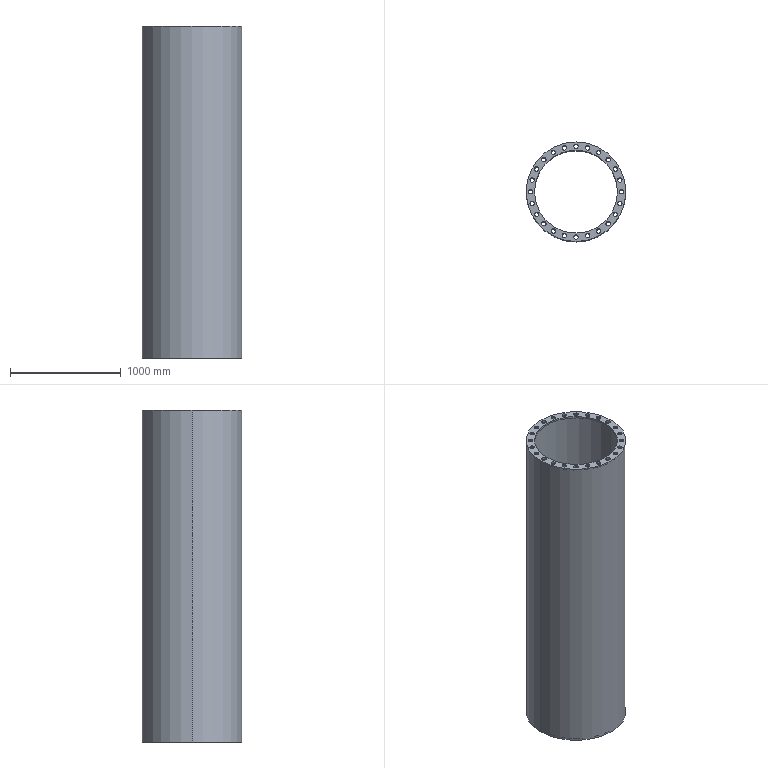Part | SolidWorks | features ICE 2, Extrusion 1, MirrorPattern 1 | 1 solid | 108 faces | box 900 x 900 x 3000 mm | volume 71509466 mm3 | cylinder 104 | plane 4 | commonest cylinder face diameters 40 x96 750 x4 884 x2 900 x2